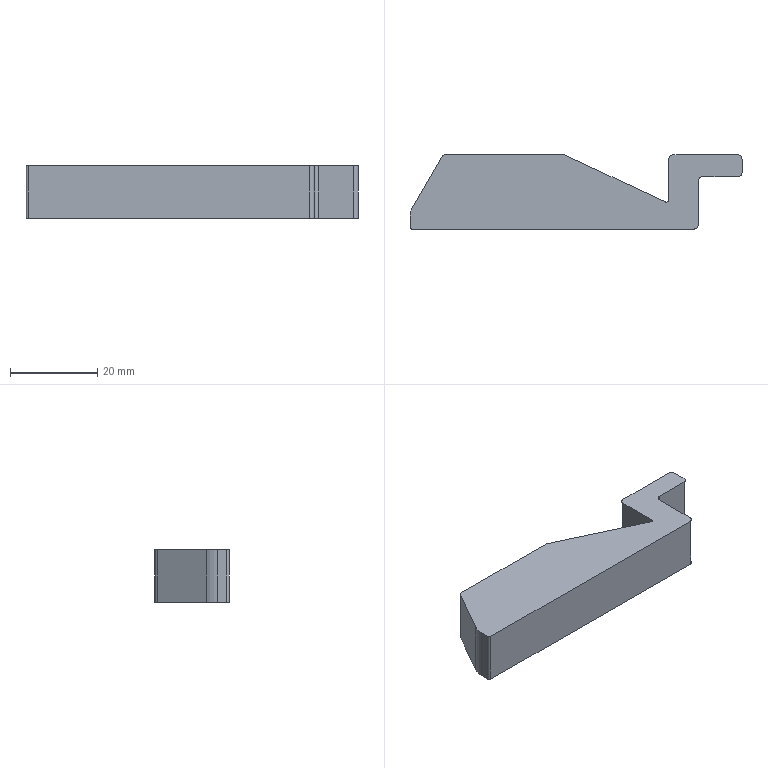Part | STEP file | con truot | 1 solid | 21 faces | box 76 x 17 x 12 mm | volume 11883 mm3 | plane 12 | cylinder 9 | commonest cylinder face diameters 2 x6 1 x2 10 x1